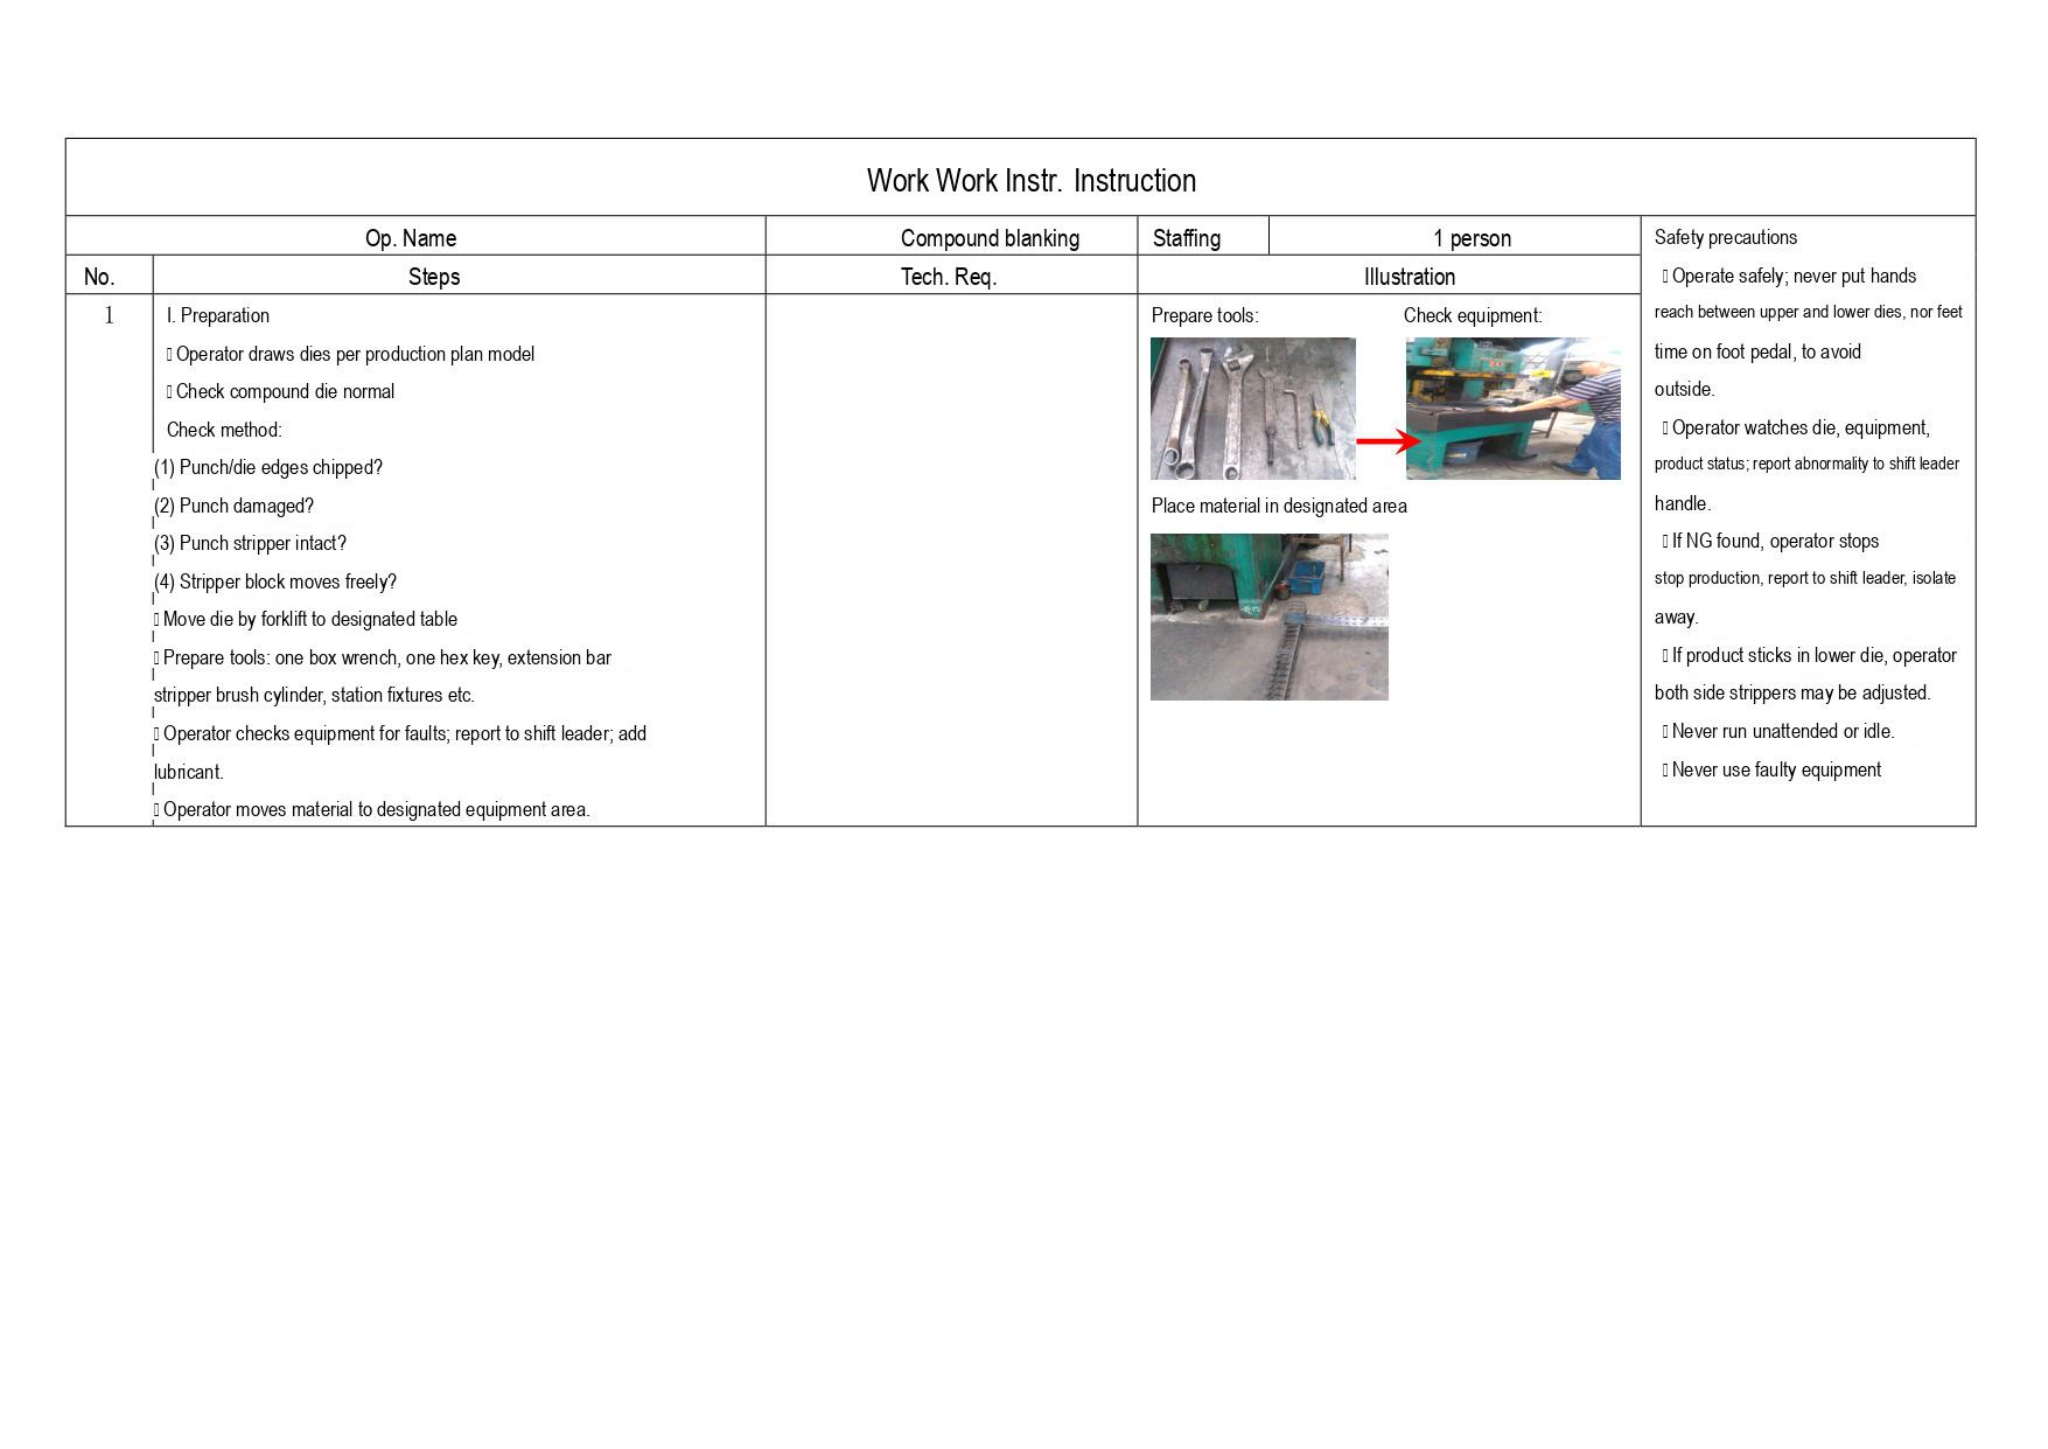Work Work Instr. Instruction

| Op. Name | | Compound blanking | Staffing | 1 person | Safety precautions |
|---|---|---|---|---|---|
| **No.** | **Steps** | **Tech. Req.** | **Illustration** | | Operate safely; never put hands reach between upper and lower dies, nor feet time on foot pedal, to avoid outside.<br>Operator watches die, equipment, product status; report abnormality to shift leader handle.<br>If NG found, operator stops stop production, report to shift leader, isolate away.<br>If product sticks in lower die, operator both side strippers may be adjusted.<br>Never run unattended or idle.<br>Never use faulty equipment |
| 1 | I. Preparation<br>Operator draws dies per production plan model<br>Check compound die normal<br>Check method:<br>(1) Punch/die edges chipped?<br>(2) Punch damaged?<br>(3) Punch stripper intact?<br>(4) Stripper block moves freely?<br>Move die by forklift to designated table<br>Prepare tools: one box wrench, one hex key, extension bar stripper brush cylinder, station fixtures etc.<br>Operator checks equipment for faults; report to shift leader; add lubricant.<br>Operator moves material to designated equipment area. | | Prepare tools:<br>Check equipment:<br>Place material in designated area | | |
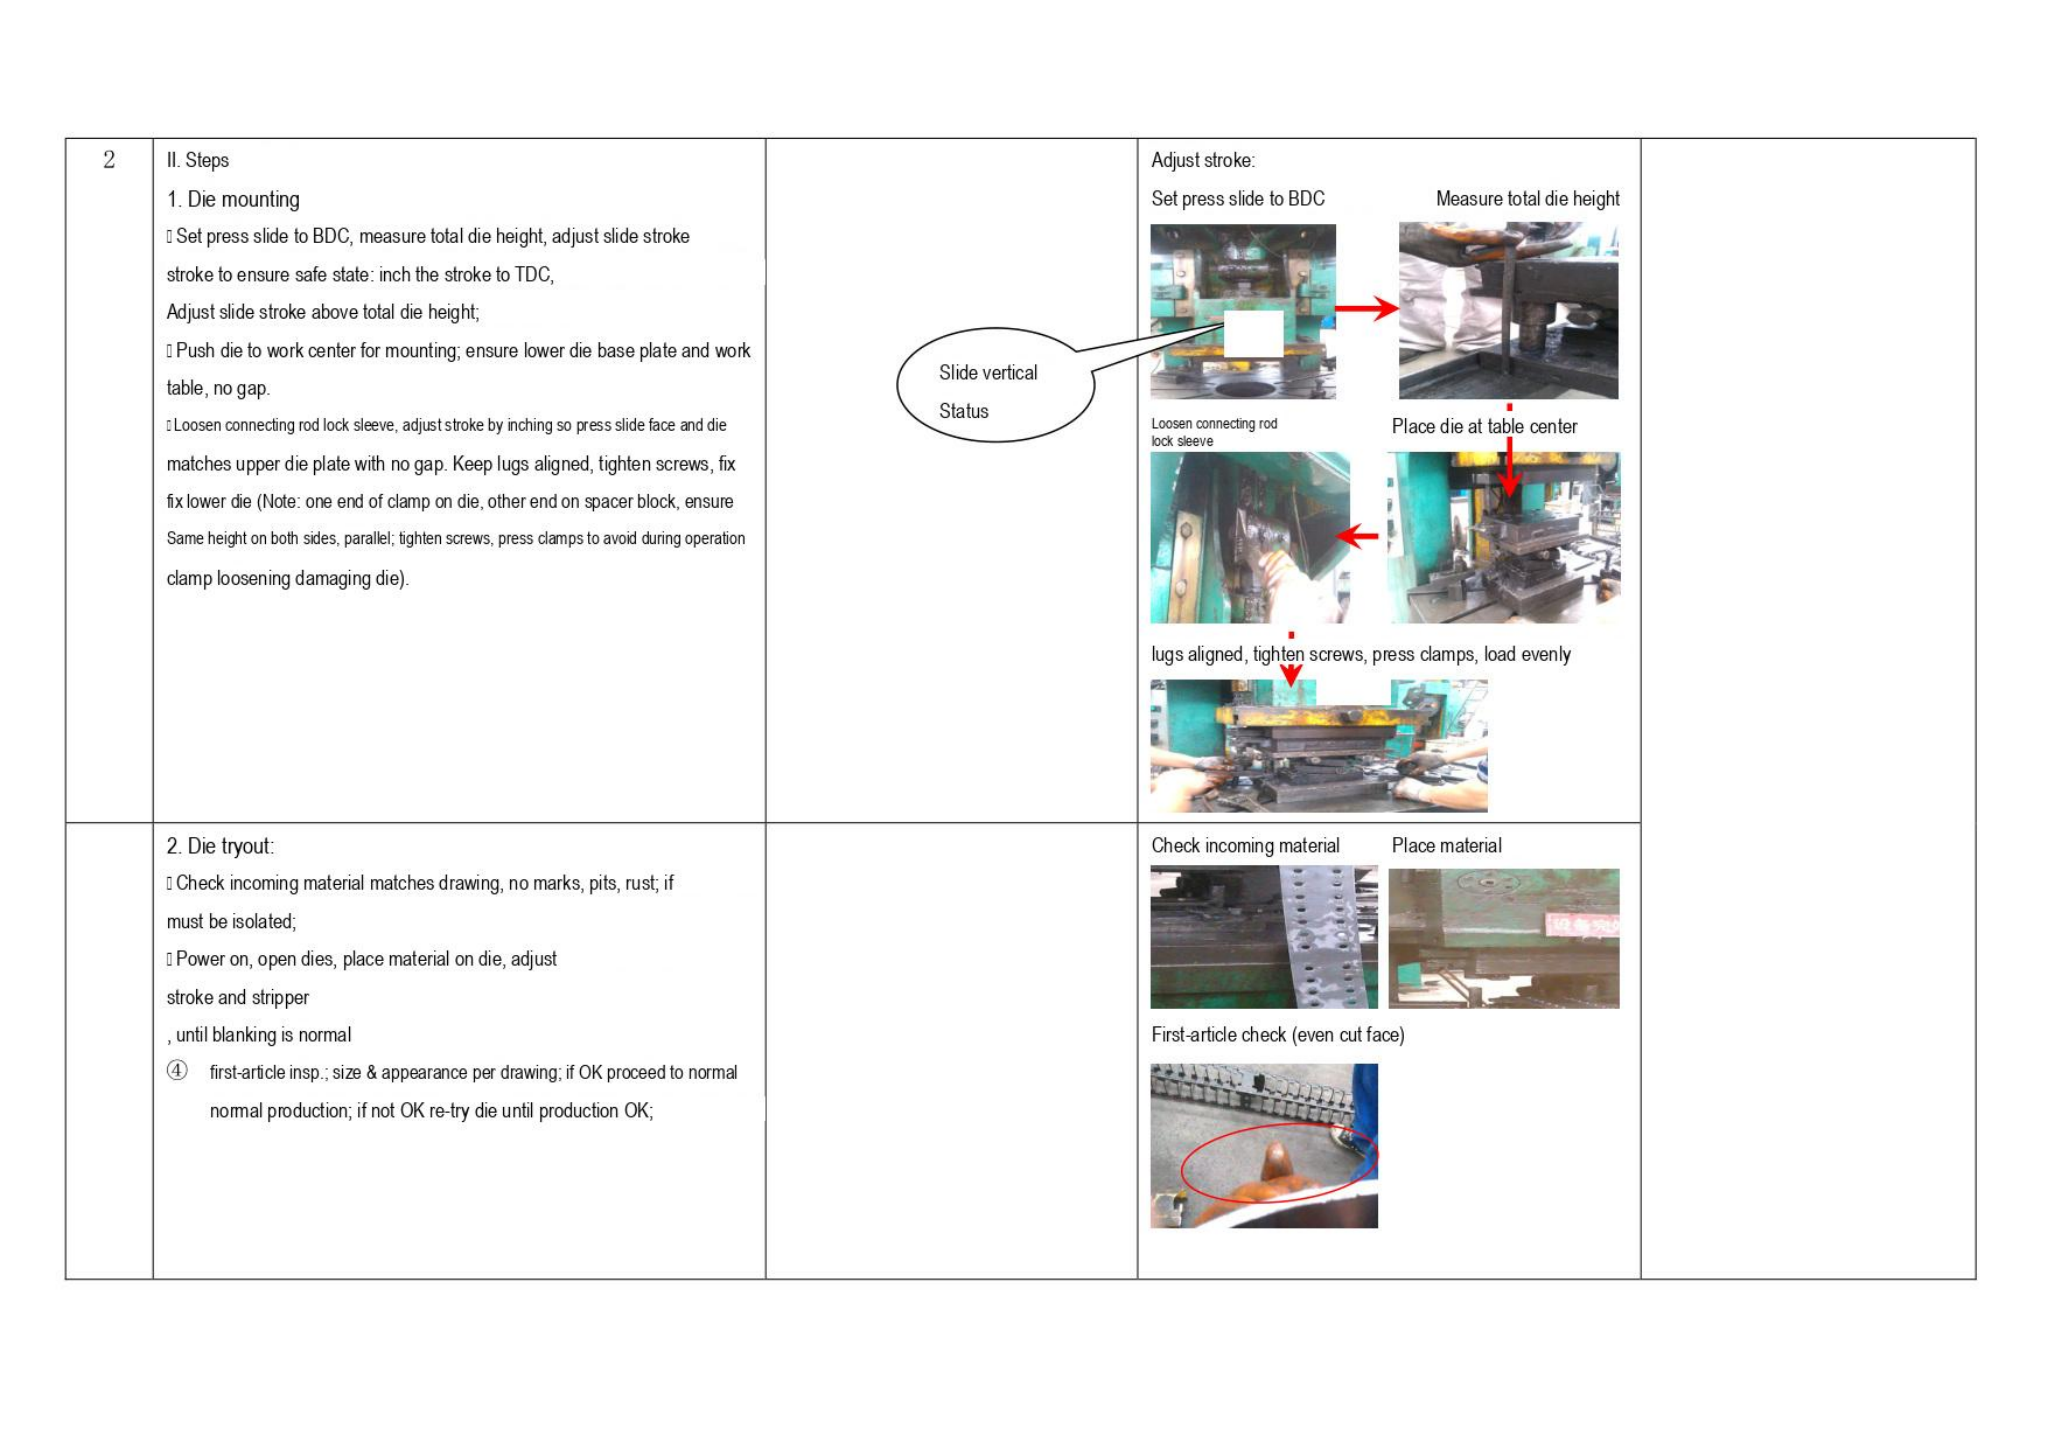| | | | | |
|---|---|---|---|---|
| 2 | II. Steps<br>1. Die mounting<br>▯ Set press slide to BDC, measure total die height, adjust slide stroke stroke to ensure safe state: inch the stroke to TDC,<br>Adjust slide stroke above total die height;<br>▯ Push die to work center for mounting; ensure lower die base plate and work table, no gap.<br>▯ Loosen connecting rod lock sleeve, adjust stroke by inching so press slide face and die matches upper die plate with no gap. Keep lugs aligned, tighten screws, fix fix lower die (Note: one end of clamp on die, other end on spacer block, ensure Same height on both sides, parallel; tighten screws, press clamps to avoid during operation clamp loosening damaging die). | Slide vertical<br>Status | Adjust stroke:<br>Set press slide to BDC<br>Measure total die height<br>Loosen connecting rod lock sleeve<br>Place die at table center<br>lugs aligned, tighten screws, press clamps, load evenly | |
| | 2. Die tryout:<br>▯ Check incoming material matches drawing, no marks, pits, rust; if must be isolated;<br>▯ Power on, open dies, place material on die, adjust stroke and stripper<br>, until blanking is normal<br>④ first-article insp.; size & appearance per drawing; if OK proceed to normal normal production; if not OK re-try die until production OK; | | Check incoming material<br>Place material<br>First-article check (even cut face) | |
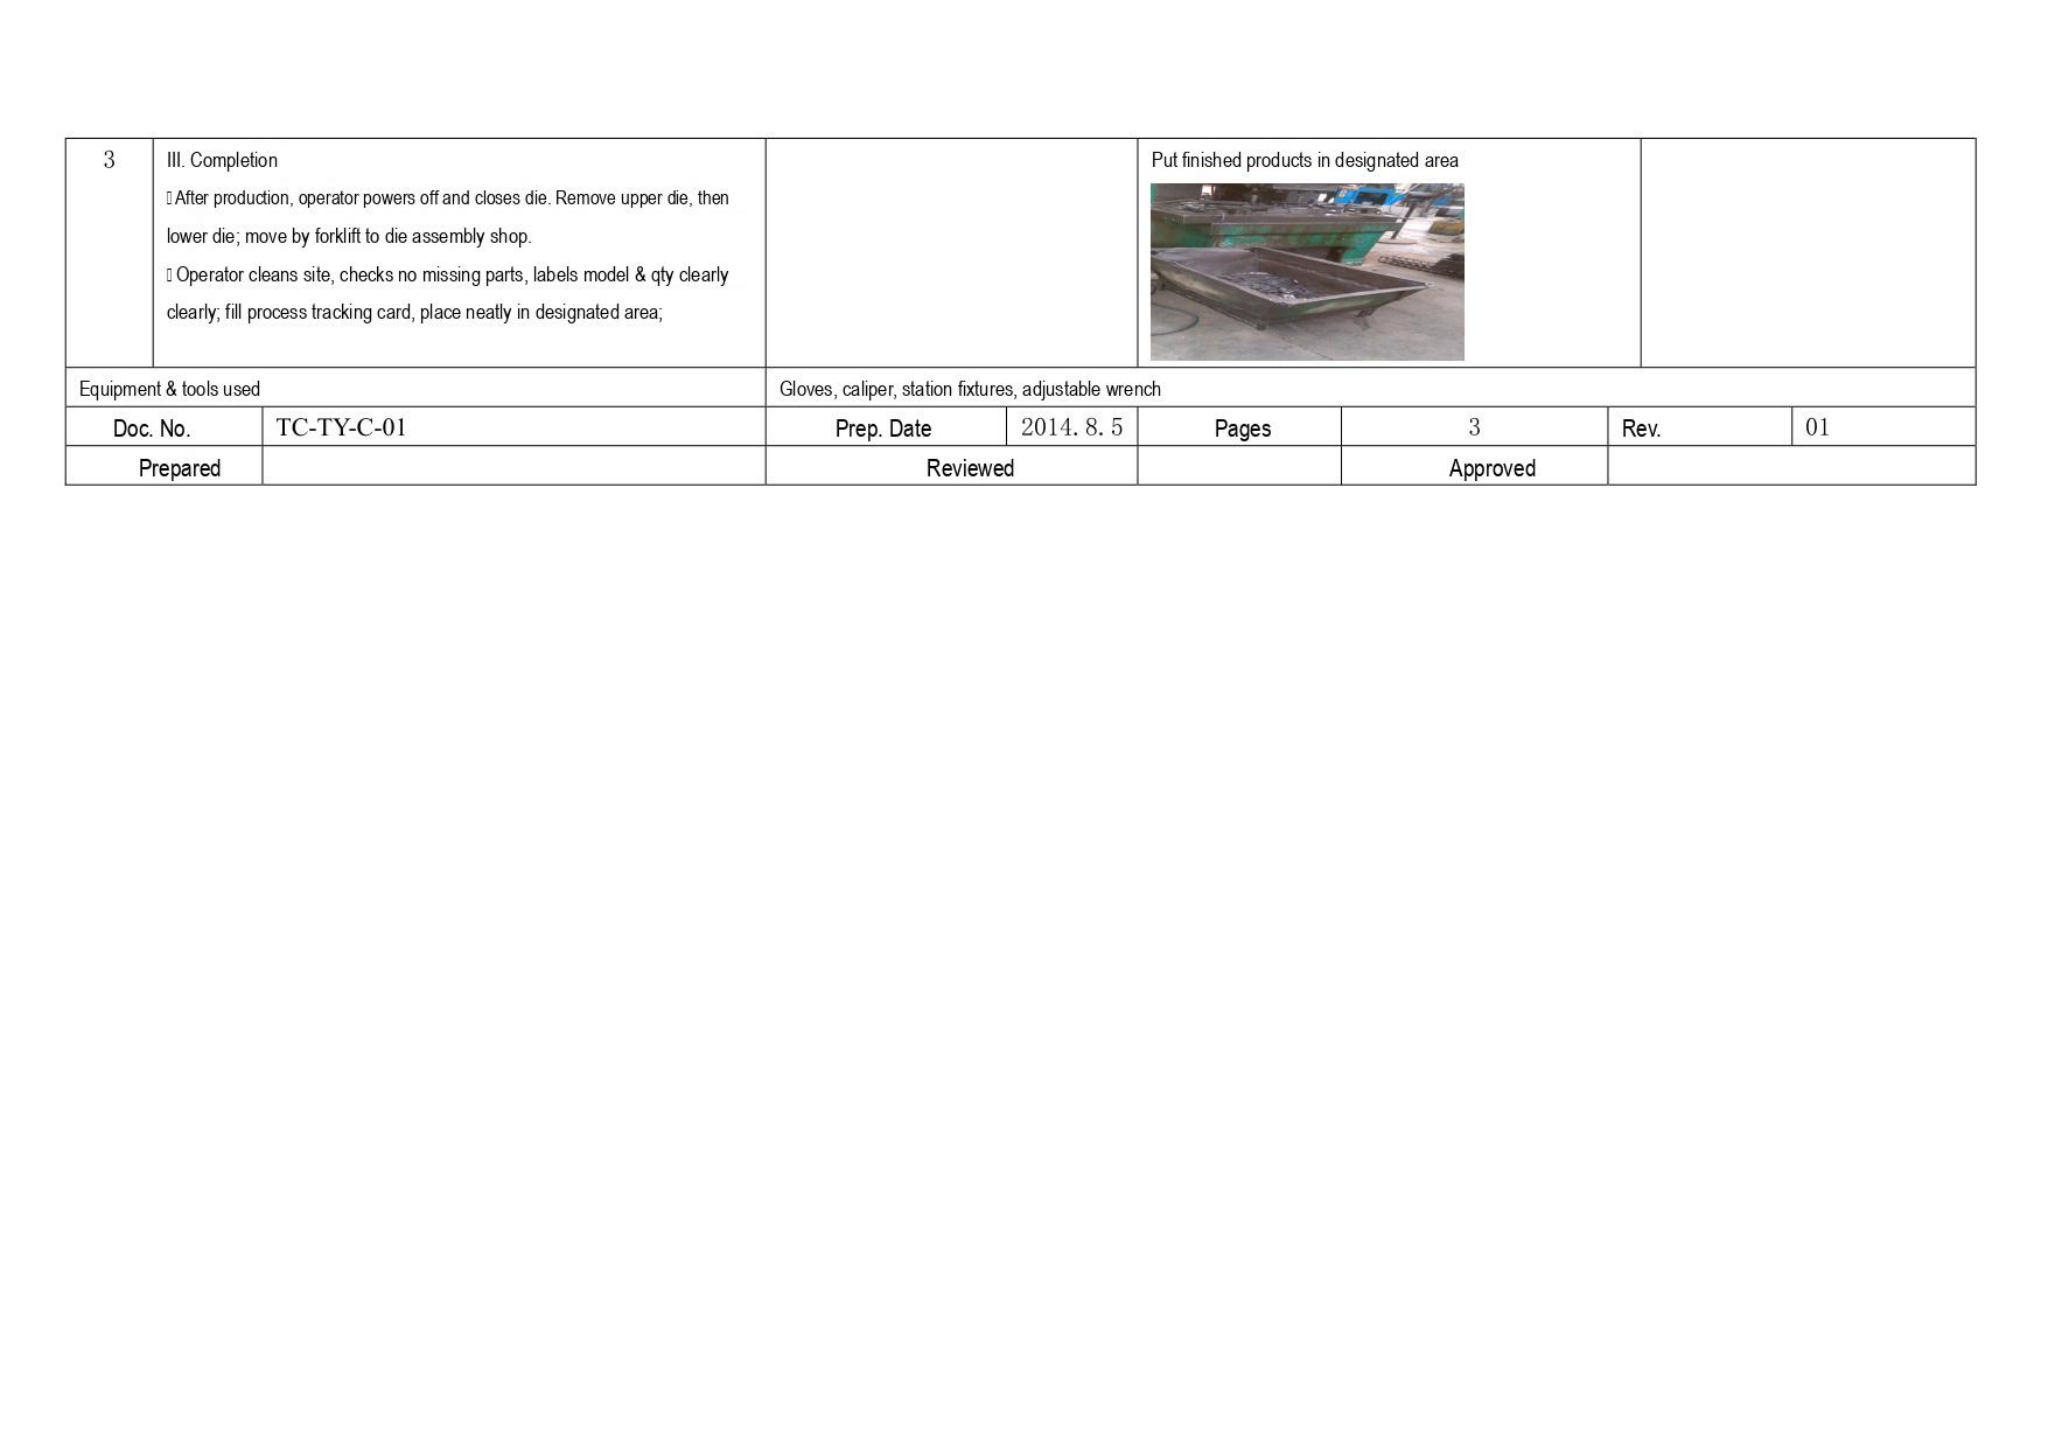| 3 | III. Completion<br>After production, operator powers off and closes die. Remove upper die, then lower die; move by forklift to die assembly shop.<br>Operator cleans site, checks no missing parts, labels model & qty clearly clearly; fill process tracking card, place neatly in designated area; | | Put finished products in designated area | |
|---|---|---|---|---|
| Equipment & tools used | | Gloves, caliper, station fixtures, adjustable wrench | | |

| Doc. No. | TC-TY-C-01 | Prep. Date | 2014. 8. 5 | Pages | 3 | Rev. | 01 |
|---|---|---|---|---|---|---|---|
| Prepared | | Reviewed | | Approved | | | |